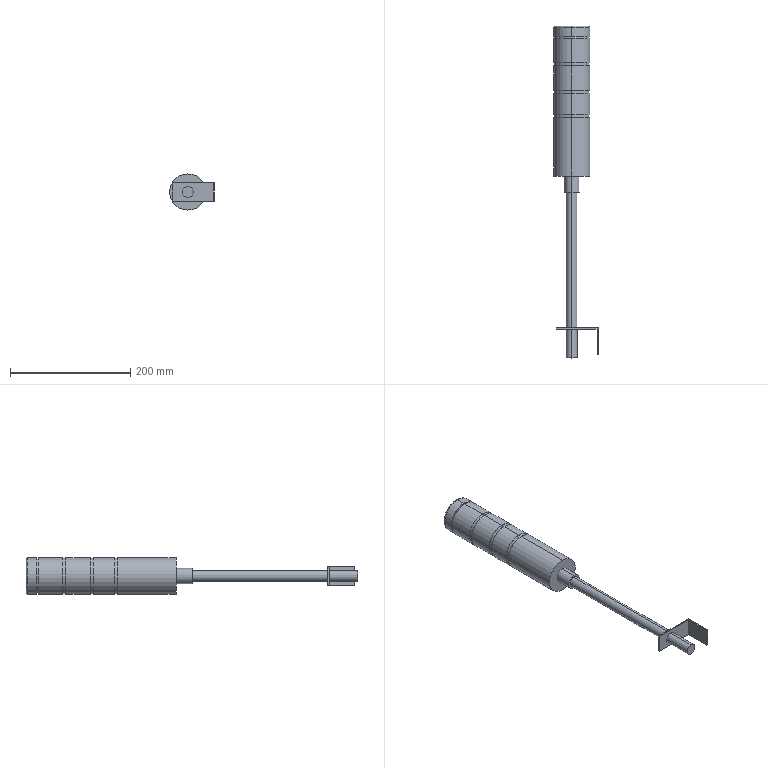Part | SolidWorks | features Boss 11, ICE 3, BossThin 1, Cut 1, Fillet 1, Shell 1, Sweep 1 | 1 solid | 46 faces | box 74 x 551.1 x 60 mm | volume 791689 mm3 | cylinder 24 | plane 20 | torus 2 | commonest cylinder face diameters 60 x10 59 x6 18 x4 25 x2 58 x2
STEP:
#1=CARTESIAN_POINT('',(212.5,682.5,-84.));
#2=VERTEX_POINT('',#1);
#3=CARTESIAN_POINT('',(212.5,682.5,-66.));
#4=VERTEX_POINT('',#3);
#5=CARTESIAN_POINT('',(212.5,682.5,-75.));
#6=DIRECTION('',(0.,-1.,0.));
#7=DIRECTION('',(0.,0.,-1.));
#8=AXIS2_PLACEMENT_3D('',#5,#6,#7);
#9=CIRCLE('',#8,9.);
#10=EDGE_CURVE('',#2,#4,#9,.T.);
#11=ORIENTED_EDGE('',*,*,#10,.F.);
#12=CARTESIAN_POINT('',(212.5,730.5,-84.));
#13=VERTEX_POINT('',#12);
#14=CARTESIAN_POINT('',(212.5,682.5,-84.));
#15=DIRECTION('',(0.,1.,0.));
#16=VECTOR('',#15,1000.);
#17=LINE('',#14,#16);
#18=EDGE_CURVE('',#2,#13,#17,.T.);
#19=ORIENTED_EDGE('',*,*,#18,.T.);
#20=CARTESIAN_POINT('',(212.5,730.5,-66.));
#21=VERTEX_POINT('',#20);
#22=CARTESIAN_POINT('',(212.5,730.5,-75.));
#23=DIRECTION('',(0.,1.,0.));
#24=DIRECTION('',(0.,0.,1.));
#25=AXIS2_PLACEMENT_3D('',#22,#23,#24);
#26=CIRCLE('',#25,9.);
#27=EDGE_CURVE('',#21,#13,#26,.T.);
#28=ORIENTED_EDGE('',*,*,#27,.F.);
#29=CARTESIAN_POINT('',(212.5,682.5,-66.));
#30=DIRECTION('',(0.,1.,0.));
#31=VECTOR('',#30,1000.);
#32=LINE('',#29,#31);
#33=EDGE_CURVE('',#4,#21,#32,.T.);
#34=ORIENTED_EDGE('',*,*,#33,.F.);
#35=EDGE_LOOP('',(#11,#19,#28,#34));
#36=FACE_OUTER_BOUND('',#35,.T.);
#37=CARTESIAN_POINT('',(212.5,682.5,-75.));
#38=DIRECTION('',(0.,1.,0.));
#39=DIRECTION('',(0.,0.,1.));
#40=AXIS2_PLACEMENT_3D('',#37,#38,#39);
#41=CYLINDRICAL_SURFACE('',#40,9.);
#42=ADVANCED_FACE('',(#36),#41,.T.);
#43=CARTESIAN_POINT('',(212.5,732.5,-66.));
#44=VERTEX_POINT('',#43);
#45=CARTESIAN_POINT('',(212.5,732.5,-84.));
#46=VERTEX_POINT('',#45);
#47=CARTESIAN_POINT('',(212.5,732.5,-75.));
#48=DIRECTION('',(0.,1.,0.));
#49=DIRECTION('',(0.,0.,1.));
#50=AXIS2_PLACEMENT_3D('',#47,#48,#49);
#51=CIRCLE('',#50,9.);
#52=EDGE_CURVE('',#44,#46,#51,.T.);
#53=ORIENTED_EDGE('',*,*,#52,.T.);
#54=CARTESIAN_POINT('',(212.5,957.5,-84.));
#55=VERTEX_POINT('',#54);
#56=CARTESIAN_POINT('',(212.5,682.5,-84.));
#57=DIRECTION('',(0.,1.,0.));
#58=VECTOR('',#57,1000.);
#59=LINE('',#56,#58);
#60=EDGE_CURVE('',#46,#55,#59,.T.);
#61=ORIENTED_EDGE('',*,*,#60,.T.);
#62=CARTESIAN_POINT('',(212.5,957.5,-66.));
#63=VERTEX_POINT('',#62);
#64=CARTESIAN_POINT('',(212.5,957.5,-75.));
#65=DIRECTION('',(0.,-1.,0.));
#66=DIRECTION('',(0.,0.,-1.));
#67=AXIS2_PLACEMENT_3D('',#64,#65,#66);
#68=CIRCLE('',#67,9.);
#69=EDGE_CURVE('',#55,#63,#68,.T.);
#70=ORIENTED_EDGE('',*,*,#69,.T.);
#71=CARTESIAN_POINT('',(212.5,682.5,-66.));
#72=DIRECTION('',(0.,1.,0.));
#73=VECTOR('',#72,1000.);
#74=LINE('',#71,#73);
#75=EDGE_CURVE('',#44,#63,#74,.T.);
#76=ORIENTED_EDGE('',*,*,#75,.F.);
#77=EDGE_LOOP('',(#53,#61,#70,#76));
#78=FACE_OUTER_BOUND('',#77,.T.);
#79=CARTESIAN_POINT('',(212.5,682.5,-75.));
#80=DIRECTION('',(0.,1.,0.));
#81=DIRECTION('',(0.,0.,1.));
#82=AXIS2_PLACEMENT_3D('',#79,#80,#81);
#83=CYLINDRICAL_SURFACE('',#82,9.);
#84=ADVANCED_FACE('',(#78),#83,.T.);
#85=CARTESIAN_POINT('',(212.5,957.5,-87.5));
#86=VERTEX_POINT('',#85);
#87=CARTESIAN_POINT('',(212.5,957.5,-62.5));
#88=VERTEX_POINT('',#87);
#89=CARTESIAN_POINT('',(212.5,957.5,-75.));
#90=DIRECTION('',(0.,-1.,0.));
#91=DIRECTION('',(0.,0.,-1.));
#92=AXIS2_PLACEMENT_3D('',#89,#90,#91);
#93=CIRCLE('',#92,12.5);
#94=EDGE_CURVE('',#86,#88,#93,.T.);
#95=ORIENTED_EDGE('',*,*,#94,.F.);
#96=CARTESIAN_POINT('',(212.5,984.5,-87.5));
#97=VERTEX_POINT('',#96);
#98=CARTESIAN_POINT('',(212.5,957.5,-87.5));
#99=DIRECTION('',(0.,1.,0.));
#100=VECTOR('',#99,1000.);
#101=LINE('',#98,#100);
#102=EDGE_CURVE('',#86,#97,#101,.T.);
#103=ORIENTED_EDGE('',*,*,#102,.T.);
#104=CARTESIAN_POINT('',(212.5,984.5,-62.5));
#105=VERTEX_POINT('',#104);
#106=CARTESIAN_POINT('',(212.5,984.5,-75.));
#107=DIRECTION('',(0.,-1.,0.));
#108=DIRECTION('',(0.,0.,1.));
#109=AXIS2_PLACEMENT_3D('',#106,#107,#108);
#110=CIRCLE('',#109,12.5);
#111=EDGE_CURVE('',#97,#105,#110,.T.);
#112=ORIENTED_EDGE('',*,*,#111,.T.);
#113=CARTESIAN_POINT('',(212.5,957.5,-62.5));
#114=DIRECTION('',(0.,1.,0.));
#115=VECTOR('',#114,1000.);
#116=LINE('',#113,#115);
#117=EDGE_CURVE('',#88,#105,#116,.T.);
#118=ORIENTED_EDGE('',*,*,#117,.F.);
#119=EDGE_LOOP('',(#95,#103,#112,#118));
#120=FACE_OUTER_BOUND('',#119,.T.);
#121=CARTESIAN_POINT('',(212.5,957.5,-75.));
#122=DIRECTION('',(0.,1.,0.));
#123=DIRECTION('',(0.,0.,1.));
#124=AXIS2_PLACEMENT_3D('',#121,#122,#123);
#125=CYLINDRICAL_SURFACE('',#124,12.5);
#126=ADVANCED_FACE('',(#120),#125,.T.);
#127=CARTESIAN_POINT('',(212.5,1230.6,-105.));
#128=VERTEX_POINT('',#127);
#129=CARTESIAN_POINT('',(212.5,1230.6,-45.));
#130=VERTEX_POINT('',#129);
#131=CARTESIAN_POINT('',(212.5,1230.6,-75.));
#132=DIRECTION('',(0.,-1.,0.));
#133=DIRECTION('',(0.,0.,1.));
#134=AXIS2_PLACEMENT_3D('',#131,#132,#133);
#135=CIRCLE('',#134,30.);
#136=EDGE_CURVE('',#128,#130,#135,.T.);
#137=ORIENTED_EDGE('',*,*,#136,.F.);
#138=CARTESIAN_POINT('',(212.5,1233.6,-102.));
#139=VERTEX_POINT('',#138);
#140=CARTESIAN_POINT('',(212.5,1230.6,-102.));
#141=DIRECTION('',(1.,0.,0.));
#142=DIRECTION('',(0.,0.,-1.));
#143=AXIS2_PLACEMENT_3D('',#140,#141,#142);
#144=CIRCLE('',#143,3.);
#145=EDGE_CURVE('',#128,#139,#144,.T.);
#146=ORIENTED_EDGE('',*,*,#145,.T.);
#147=CARTESIAN_POINT('',(212.5,1233.6,-48.));
#148=VERTEX_POINT('',#147);
#149=CARTESIAN_POINT('',(212.5,1233.6,-75.));
#150=DIRECTION('',(0.,1.,0.));
#151=DIRECTION('',(0.,0.,1.));
#152=AXIS2_PLACEMENT_3D('',#149,#150,#151);
#153=CIRCLE('',#152,27.);
#154=EDGE_CURVE('',#148,#139,#153,.T.);
#155=ORIENTED_EDGE('',*,*,#154,.F.);
#156=CARTESIAN_POINT('',(212.5,1230.6,-48.));
#157=DIRECTION('',(-1.,0.,0.));
#158=DIRECTION('',(0.,-1.,0.));
#159=AXIS2_PLACEMENT_3D('',#156,#157,#158);
#160=CIRCLE('',#159,3.);
#161=EDGE_CURVE('',#130,#148,#160,.T.);
#162=ORIENTED_EDGE('',*,*,#161,.F.);
#163=EDGE_LOOP('',(#137,#146,#155,#162));
#164=FACE_OUTER_BOUND('',#163,.T.);
#165=CARTESIAN_POINT('',(212.5,1230.6,-75.));
#166=DIRECTION('',(0.,1.,0.));
#167=DIRECTION('',(0.,0.,1.));
#168=AXIS2_PLACEMENT_3D('',#165,#166,#167);
#169=TOROIDAL_SURFACE('',#168,27.,3.);
#170=ADVANCED_FACE('',(#164),#169,.T.);
#171=ORIENTED_EDGE('',*,*,#136,.T.);
#172=CARTESIAN_POINT('',(212.5,1215.6,-45.));
#173=VERTEX_POINT('',#172);
#174=CARTESIAN_POINT('',(212.5,1233.6,-45.));
#175=DIRECTION('',(0.,-1.,0.));
#176=VECTOR('',#175,1000.);
#177=LINE('',#174,#176);
#178=EDGE_CURVE('',#130,#173,#177,.T.);
#179=ORIENTED_EDGE('',*,*,#178,.T.);
#180=CARTESIAN_POINT('',(212.5,1215.6,-105.));
#181=VERTEX_POINT('',#180);
#182=CARTESIAN_POINT('',(212.5,1215.6,-75.));
#183=DIRECTION('',(0.,1.,0.));
#184=DIRECTION('',(0.,0.,1.));
#185=AXIS2_PLACEMENT_3D('',#182,#183,#184);
#186=CIRCLE('',#185,30.);
#187=EDGE_CURVE('',#173,#181,#186,.T.);
#188=ORIENTED_EDGE('',*,*,#187,.T.);
#189=CARTESIAN_POINT('',(212.5,1233.6,-105.));
#190=DIRECTION('',(0.,-1.,0.));
#191=VECTOR('',#190,1000.);
#192=LINE('',#189,#191);
#193=EDGE_CURVE('',#128,#181,#192,.T.);
#194=ORIENTED_EDGE('',*,*,#193,.F.);
#195=EDGE_LOOP('',(#171,#179,#188,#194));
#196=FACE_OUTER_BOUND('',#195,.T.);
#197=CARTESIAN_POINT('',(212.5,1233.6,-75.));
#198=DIRECTION('',(0.,-1.,0.));
#199=DIRECTION('',(0.,0.,-1.));
#200=AXIS2_PLACEMENT_3D('',#197,#198,#199);
#201=CYLINDRICAL_SURFACE('',#200,30.);
#202=ADVANCED_FACE('',(#196),#201,.T.);
#203=CARTESIAN_POINT('',(212.5,1215.6,-46.));
#204=VERTEX_POINT('',#203);
#205=CARTESIAN_POINT('',(212.5,1215.6,-104.));
#206=VERTEX_POINT('',#205);
#207=CARTESIAN_POINT('',(212.5,1215.6,-75.));
#208=DIRECTION('',(0.,1.,0.));
#209=DIRECTION('',(0.,0.,1.));
#210=AXIS2_PLACEMENT_3D('',#207,#208,#209);
#211=CIRCLE('',#210,29.);
#212=EDGE_CURVE('',#204,#206,#211,.T.);
#213=ORIENTED_EDGE('',*,*,#212,.F.);
#214=CARTESIAN_POINT('',(212.5,1213.6,-46.));
#215=VERTEX_POINT('',#214);
#216=CARTESIAN_POINT('',(212.5,1215.6,-46.));
#217=DIRECTION('',(0.,-1.,0.));
#218=VECTOR('',#217,1000.);
#219=LINE('',#216,#218);
#220=EDGE_CURVE('',#204,#215,#219,.T.);
#221=ORIENTED_EDGE('',*,*,#220,.T.);
#222=CARTESIAN_POINT('',(212.5,1213.6,-104.));
#223=VERTEX_POINT('',#222);
#224=CARTESIAN_POINT('',(212.5,1213.6,-75.));
#225=DIRECTION('',(0.,1.,0.));
#226=DIRECTION('',(0.,0.,1.));
#227=AXIS2_PLACEMENT_3D('',#224,#225,#226);
#228=CIRCLE('',#227,29.);
#229=EDGE_CURVE('',#215,#223,#228,.T.);
#230=ORIENTED_EDGE('',*,*,#229,.T.);
#231=CARTESIAN_POINT('',(212.5,1215.6,-104.));
#232=DIRECTION('',(0.,-1.,0.));
#233=VECTOR('',#232,1000.);
#234=LINE('',#231,#233);
#235=EDGE_CURVE('',#206,#223,#234,.T.);
#236=ORIENTED_EDGE('',*,*,#235,.F.);
#237=EDGE_LOOP('',(#213,#221,#230,#236));
#238=FACE_OUTER_BOUND('',#237,.T.);
#239=CARTESIAN_POINT('',(212.5,1215.6,-75.));
#240=DIRECTION('',(0.,-1.,0.));
#241=DIRECTION('',(0.,0.,-1.));
#242=AXIS2_PLACEMENT_3D('',#239,#240,#241);
#243=CYLINDRICAL_SURFACE('',#242,29.);
#244=ADVANCED_FACE('',(#238),#243,.T.);
#245=CARTESIAN_POINT('',(212.5,1213.6,-45.));
#246=VERTEX_POINT('',#245);
#247=CARTESIAN_POINT('',(212.5,1213.6,-105.));
#248=VERTEX_POINT('',#247);
#249=CARTESIAN_POINT('',(212.5,1213.6,-75.));
#250=DIRECTION('',(0.,1.,0.));
#251=DIRECTION('',(0.,0.,1.));
#252=AXIS2_PLACEMENT_3D('',#249,#250,#251);
#253=CIRCLE('',#252,30.);
#254=EDGE_CURVE('',#246,#248,#253,.T.);
#255=ORIENTED_EDGE('',*,*,#254,.F.);
#256=CARTESIAN_POINT('',(212.5,1172.6,-45.));
#257=VERTEX_POINT('',#256);
#258=CARTESIAN_POINT('',(212.5,1213.6,-45.));
#259=DIRECTION('',(0.,-1.,0.));
#260=VECTOR('',#259,1000.);
#261=LINE('',#258,#260);
#262=EDGE_CURVE('',#246,#257,#261,.T.);
#263=ORIENTED_EDGE('',*,*,#262,.T.);
#264=CARTESIAN_POINT('',(212.5,1172.6,-105.));
#265=VERTEX_POINT('',#264);
#266=CARTESIAN_POINT('',(212.5,1172.6,-75.));
#267=DIRECTION('',(0.,1.,0.));
#268=DIRECTION('',(0.,0.,1.));
#269=AXIS2_PLACEMENT_3D('',#266,#267,#268);
#270=CIRCLE('',#269,30.);
#271=EDGE_CURVE('',#257,#265,#270,.T.);
#272=ORIENTED_EDGE('',*,*,#271,.T.);
#273=CARTESIAN_POINT('',(212.5,1213.6,-105.));
#274=DIRECTION('',(0.,-1.,0.));
#275=VECTOR('',#274,1000.);
#276=LINE('',#273,#275);
#277=EDGE_CURVE('',#248,#265,#276,.T.);
#278=ORIENTED_EDGE('',*,*,#277,.F.);
#279=EDGE_LOOP('',(#255,#263,#272,#278));
#280=FACE_OUTER_BOUND('',#279,.T.);
#281=CARTESIAN_POINT('',(212.5,1213.6,-75.));
#282=DIRECTION('',(0.,-1.,0.));
#283=DIRECTION('',(0.,0.,-1.));
#284=AXIS2_PLACEMENT_3D('',#281,#282,#283);
#285=CYLINDRICAL_SURFACE('',#284,30.);
#286=ADVANCED_FACE('',(#280),#285,.T.);
#287=CARTESIAN_POINT('',(212.5,1172.6,-45.5));
#288=VERTEX_POINT('',#287);
#289=CARTESIAN_POINT('',(212.5,1172.6,-104.5));
#290=VERTEX_POINT('',#289);
#291=CARTESIAN_POINT('',(212.5,1172.6,-75.));
#292=DIRECTION('',(0.,1.,0.));
#293=DIRECTION('',(0.,0.,1.));
#294=AXIS2_PLACEMENT_3D('',#291,#292,#293);
#295=CIRCLE('',#294,29.5);
#296=EDGE_CURVE('',#288,#290,#295,.T.);
#297=ORIENTED_EDGE('',*,*,#296,.F.);
#298=CARTESIAN_POINT('',(212.5,1167.6,-45.5));
#299=VERTEX_POINT('',#298);
#300=CARTESIAN_POINT('',(212.5,1172.6,-45.5));
#301=DIRECTION('',(0.,-1.,0.));
#302=VECTOR('',#301,1000.);
#303=LINE('',#300,#302);
#304=EDGE_CURVE('',#288,#299,#303,.T.);
#305=ORIENTED_EDGE('',*,*,#304,.T.);
#306=CARTESIAN_POINT('',(212.5,1167.6,-104.5));
#307=VERTEX_POINT('',#306);
#308=CARTESIAN_POINT('',(212.5,1167.6,-75.));
#309=DIRECTION('',(0.,1.,0.));
#310=DIRECTION('',(0.,0.,1.));
#311=AXIS2_PLACEMENT_3D('',#308,#309,#310);
#312=CIRCLE('',#311,29.5);
#313=EDGE_CURVE('',#299,#307,#312,.T.);
#314=ORIENTED_EDGE('',*,*,#313,.T.);
#315=CARTESIAN_POINT('',(212.5,1172.6,-104.5));
#316=DIRECTION('',(0.,-1.,0.));
#317=VECTOR('',#316,1000.);
#318=LINE('',#315,#317);
#319=EDGE_CURVE('',#290,#307,#318,.T.);
#320=ORIENTED_EDGE('',*,*,#319,.F.);
#321=EDGE_LOOP('',(#297,#305,#314,#320));
#322=FACE_OUTER_BOUND('',#321,.T.);
#323=CARTESIAN_POINT('',(212.5,1172.6,-75.));
#324=DIRECTION('',(0.,-1.,0.));
#325=DIRECTION('',(0.,0.,-1.));
#326=AXIS2_PLACEMENT_3D('',#323,#324,#325);
#327=CYLINDRICAL_SURFACE('',#326,29.5);
#328=ADVANCED_FACE('',(#322),#327,.T.);
#329=CARTESIAN_POINT('',(212.5,1167.6,-45.));
#330=VERTEX_POINT('',#329);
#331=CARTESIAN_POINT('',(212.5,1167.6,-105.));
#332=VERTEX_POINT('',#331);
#333=CARTESIAN_POINT('',(212.5,1167.6,-75.));
#334=DIRECTION('',(0.,1.,0.));
#335=DIRECTION('',(0.,0.,1.));
#336=AXIS2_PLACEMENT_3D('',#333,#334,#335);
#337=CIRCLE('',#336,30.);
#338=EDGE_CURVE('',#330,#332,#337,.T.);
#339=ORIENTED_EDGE('',*,*,#338,.F.);
#340=CARTESIAN_POINT('',(212.5,1126.6,-45.));
#341=VERTEX_POINT('',#340);
#342=CARTESIAN_POINT('',(212.5,1167.6,-45.));
#343=DIRECTION('',(0.,-1.,0.));
#344=VECTOR('',#343,1000.);
#345=LINE('',#342,#344);
#346=EDGE_CURVE('',#330,#341,#345,.T.);
#347=ORIENTED_EDGE('',*,*,#346,.T.);
#348=CARTESIAN_POINT('',(212.5,1126.6,-105.));
#349=VERTEX_POINT('',#348);
#350=CARTESIAN_POINT('',(212.5,1126.6,-75.));
#351=DIRECTION('',(0.,1.,0.));
#352=DIRECTION('',(0.,0.,1.));
#353=AXIS2_PLACEMENT_3D('',#350,#351,#352);
#354=CIRCLE('',#353,30.);
#355=EDGE_CURVE('',#341,#349,#354,.T.);
#356=ORIENTED_EDGE('',*,*,#355,.T.);
#357=CARTESIAN_POINT('',(212.5,1167.6,-105.));
#358=DIRECTION('',(0.,-1.,0.));
#359=VECTOR('',#358,1000.);
#360=LINE('',#357,#359);
#361=EDGE_CURVE('',#332,#349,#360,.T.);
#362=ORIENTED_EDGE('',*,*,#361,.F.);
#363=EDGE_LOOP('',(#339,#347,#356,#362));
#364=FACE_OUTER_BOUND('',#363,.T.);
#365=CARTESIAN_POINT('',(212.5,1167.6,-75.));
#366=DIRECTION('',(0.,-1.,0.));
#367=DIRECTION('',(0.,0.,-1.));
#368=AXIS2_PLACEMENT_3D('',#365,#366,#367);
#369=CYLINDRICAL_SURFACE('',#368,30.);
#370=ADVANCED_FACE('',(#364),#369,.T.);
#371=CARTESIAN_POINT('',(212.5,1126.6,-45.5));
#372=VERTEX_POINT('',#371);
#373=CARTESIAN_POINT('',(212.5,1126.6,-104.5));
#374=VERTEX_POINT('',#373);
#375=CARTESIAN_POINT('',(212.5,1126.6,-75.));
#376=DIRECTION('',(0.,1.,0.));
#377=DIRECTION('',(0.,0.,1.));
#378=AXIS2_PLACEMENT_3D('',#375,#376,#377);
#379=CIRCLE('',#378,29.5);
#380=EDGE_CURVE('',#372,#374,#379,.T.);
#381=ORIENTED_EDGE('',*,*,#380,.F.);
#382=CARTESIAN_POINT('',(212.5,1121.6,-45.5));
#383=VERTEX_POINT('',#382);
#384=CARTESIAN_POINT('',(212.5,1126.6,-45.5));
#385=DIRECTION('',(0.,-1.,0.));
#386=VECTOR('',#385,1000.);
#387=LINE('',#384,#386);
#388=EDGE_CURVE('',#372,#383,#387,.T.);
#389=ORIENTED_EDGE('',*,*,#388,.T.);
#390=CARTESIAN_POINT('',(212.5,1121.6,-104.5));
#391=VERTEX_POINT('',#390);
#392=CARTESIAN_POINT('',(212.5,1121.6,-75.));
#393=DIRECTION('',(0.,1.,0.));
#394=DIRECTION('',(0.,0.,1.));
#395=AXIS2_PLACEMENT_3D('',#392,#393,#394);
#396=CIRCLE('',#395,29.5);
#397=EDGE_CURVE('',#383,#391,#396,.T.);
#398=ORIENTED_EDGE('',*,*,#397,.T.);
#399=CARTESIAN_POINT('',(212.5,1126.6,-104.5));
#400=DIRECTION('',(0.,-1.,0.));
#401=VECTOR('',#400,1000.);
#402=LINE('',#399,#401);
#403=EDGE_CURVE('',#374,#391,#402,.T.);
#404=ORIENTED_EDGE('',*,*,#403,.F.);
#405=EDGE_LOOP('',(#381,#389,#398,#404));
#406=FACE_OUTER_BOUND('',#405,.T.);
#407=CARTESIAN_POINT('',(212.5,1126.6,-75.));
#408=DIRECTION('',(0.,-1.,0.));
#409=DIRECTION('',(0.,0.,-1.));
#410=AXIS2_PLACEMENT_3D('',#407,#408,#409);
#411=CYLINDRICAL_SURFACE('',#410,29.5);
#412=ADVANCED_FACE('',(#406),#411,.T.);
#413=CARTESIAN_POINT('',(212.5,1121.6,-45.));
#414=VERTEX_POINT('',#413);
#415=CARTESIAN_POINT('',(212.5,1121.6,-105.));
#416=VERTEX_POINT('',#415);
#417=CARTESIAN_POINT('',(212.5,1121.6,-75.));
#418=DIRECTION('',(0.,1.,0.));
#419=DIRECTION('',(0.,0.,1.));
#420=AXIS2_PLACEMENT_3D('',#417,#418,#419);
#421=CIRCLE('',#420,30.);
#422=EDGE_CURVE('',#414,#416,#421,.T.);
#423=ORIENTED_EDGE('',*,*,#422,.F.);
#424=CARTESIAN_POINT('',(212.5,1086.6,-45.));
#425=VERTEX_POINT('',#424);
#426=CARTESIAN_POINT('',(212.5,1121.6,-45.));
#427=DIRECTION('',(0.,-1.,0.));
#428=VECTOR('',#427,1000.);
#429=LINE('',#426,#428);
#430=EDGE_CURVE('',#414,#425,#429,.T.);
#431=ORIENTED_EDGE('',*,*,#430,.T.);
#432=CARTESIAN_POINT('',(212.5,1086.6,-105.));
#433=VERTEX_POINT('',#432);
#434=CARTESIAN_POINT('',(212.5,1086.6,-75.));
#435=DIRECTION('',(0.,1.,0.));
#436=DIRECTION('',(0.,0.,1.));
#437=AXIS2_PLACEMENT_3D('',#434,#435,#436);
#438=CIRCLE('',#437,30.);
#439=EDGE_CURVE('',#425,#433,#438,.T.);
#440=ORIENTED_EDGE('',*,*,#439,.T.);
#441=CARTESIAN_POINT('',(212.5,1121.6,-105.));
#442=DIRECTION('',(0.,-1.,0.));
#443=VECTOR('',#442,1000.);
#444=LINE('',#441,#443);
#445=EDGE_CURVE('',#416,#433,#444,.T.);
#446=ORIENTED_EDGE('',*,*,#445,.F.);
#447=EDGE_LOOP('',(#423,#431,#440,#446));
#448=FACE_OUTER_BOUND('',#447,.T.);
#449=CARTESIAN_POINT('',(212.5,1121.6,-75.));
#450=DIRECTION('',(0.,-1.,0.));
#451=DIRECTION('',(0.,0.,-1.));
#452=AXIS2_PLACEMENT_3D('',#449,#450,#451);
#453=CYLINDRICAL_SURFACE('',#452,30.);
#454=ADVANCED_FACE('',(#448),#453,.T.);
#455=CARTESIAN_POINT('',(212.5,1086.6,-45.5));
#456=VERTEX_POINT('',#455);
#457=CARTESIAN_POINT('',(212.5,1086.6,-104.5));
#458=VERTEX_POINT('',#457);
#459=CARTESIAN_POINT('',(212.5,1086.6,-75.));
#460=DIRECTION('',(0.,1.,0.));
#461=DIRECTION('',(0.,0.,1.));
#462=AXIS2_PLACEMENT_3D('',#459,#460,#461);
#463=CIRCLE('',#462,29.5);
#464=EDGE_CURVE('',#456,#458,#463,.T.);
#465=ORIENTED_EDGE('',*,*,#464,.F.);
#466=CARTESIAN_POINT('',(212.5,1081.6,-45.5));
#467=VERTEX_POINT('',#466);
#468=CARTESIAN_POINT('',(212.5,1086.6,-45.5));
#469=DIRECTION('',(0.,-1.,0.));
#470=VECTOR('',#469,1000.);
#471=LINE('',#468,#470);
#472=EDGE_CURVE('',#456,#467,#471,.T.);
#473=ORIENTED_EDGE('',*,*,#472,.T.);
#474=CARTESIAN_POINT('',(212.5,1081.6,-104.5));
#475=VERTEX_POINT('',#474);
#476=CARTESIAN_POINT('',(212.5,1081.6,-75.));
#477=DIRECTION('',(0.,1.,0.));
#478=DIRECTION('',(0.,0.,1.));
#479=AXIS2_PLACEMENT_3D('',#476,#477,#478);
#480=CIRCLE('',#479,29.5);
#481=EDGE_CURVE('',#467,#475,#480,.T.);
#482=ORIENTED_EDGE('',*,*,#481,.T.);
#483=CARTESIAN_POINT('',(212.5,1086.6,-104.5));
#484=DIRECTION('',(0.,-1.,0.));
#485=VECTOR('',#484,1000.);
#486=LINE('',#483,#485);
#487=EDGE_CURVE('',#458,#475,#486,.T.);
#488=ORIENTED_EDGE('',*,*,#487,.F.);
#489=EDGE_LOOP('',(#465,#473,#482,#488));
#490=FACE_OUTER_BOUND('',#489,.T.);
#491=CARTESIAN_POINT('',(212.5,1086.6,-75.));
#492=DIRECTION('',(0.,-1.,0.));
#493=DIRECTION('',(0.,0.,-1.));
#494=AXIS2_PLACEMENT_3D('',#491,#492,#493);
#495=CYLINDRICAL_SURFACE('',#494,29.5);
#496=ADVANCED_FACE('',(#490),#495,.T.);
#497=CARTESIAN_POINT('',(212.5,1081.6,-45.));
#498=VERTEX_POINT('',#497);
#499=CARTESIAN_POINT('',(212.5,1081.6,-105.));
#500=VERTEX_POINT('',#499);
#501=CARTESIAN_POINT('',(212.5,1081.6,-75.));
#502=DIRECTION('',(0.,1.,0.));
#503=DIRECTION('',(0.,0.,1.));
#504=AXIS2_PLACEMENT_3D('',#501,#502,#503);
#505=CIRCLE('',#504,30.);
#506=EDGE_CURVE('',#498,#500,#505,.T.);
#507=ORIENTED_EDGE('',*,*,#506,.F.);
#508=CARTESIAN_POINT('',(212.5,984.5,-45.));
#509=VERTEX_POINT('',#508);
#510=CARTESIAN_POINT('',(212.5,1081.6,-45.));
#511=DIRECTION('',(0.,-1.,0.));
#512=VECTOR('',#511,1000.);
#513=LINE('',#510,#512);
#514=EDGE_CURVE('',#498,#509,#513,.T.);
#515=ORIENTED_EDGE('',*,*,#514,.T.);
#516=CARTESIAN_POINT('',(212.5,984.5,-105.));
#517=VERTEX_POINT('',#516);
#518=CARTESIAN_POINT('',(212.5,984.5,-75.));
#519=DIRECTION('',(0.,1.,0.));
#520=DIRECTION('',(0.,0.,1.));
#521=AXIS2_PLACEMENT_3D('',#518,#519,#520);
#522=CIRCLE('',#521,30.);
#523=EDGE_CURVE('',#509,#517,#522,.T.);
#524=ORIENTED_EDGE('',*,*,#523,.T.);
#525=CARTESIAN_POINT('',(212.5,1081.6,-105.));
#526=DIRECTION('',(0.,-1.,0.));
#527=VECTOR('',#526,1000.);
#528=LINE('',#525,#527);
#529=EDGE_CURVE('',#500,#517,#528,.T.);
#530=ORIENTED_EDGE('',*,*,#529,.F.);
#531=EDGE_LOOP('',(#507,#515,#524,#530));
#532=FACE_OUTER_BOUND('',#531,.T.);
#533=CARTESIAN_POINT('',(212.5,1081.6,-75.));
#534=DIRECTION('',(0.,-1.,0.));
#535=DIRECTION('',(0.,0.,-1.));
#536=AXIS2_PLACEMENT_3D('',#533,#534,#535);
#537=CYLINDRICAL_SURFACE('',#536,30.);
#538=ADVANCED_FACE('',(#532),#537,.T.);
#539=CARTESIAN_POINT('',(212.5,957.5,-75.));
#540=DIRECTION('',(0.,-1.,0.));
#541=DIRECTION('',(0.,0.,-1.));
#542=AXIS2_PLACEMENT_3D('',#539,#540,#541);
#543=CIRCLE('',#542,12.5);
#544=EDGE_CURVE('',#88,#86,#543,.T.);
#545=ORIENTED_EDGE('',*,*,#544,.T.);
#546=ORIENTED_EDGE('',*,*,#94,.T.);
#547=EDGE_LOOP('',(#545,#546));
#548=FACE_OUTER_BOUND('',#547,.T.);
#549=CARTESIAN_POINT('',(212.5,957.5,-75.));
#550=DIRECTION('',(0.,-1.,0.));
#551=DIRECTION('',(0.,0.,-1.));
#552=AXIS2_PLACEMENT_3D('',#549,#550,#551);
#553=CIRCLE('',#552,9.);
#554=EDGE_CURVE('',#63,#55,#553,.T.);
#555=ORIENTED_EDGE('',*,*,#554,.F.);
#556=ORIENTED_EDGE('',*,*,#69,.F.);
#557=EDGE_LOOP('',(#555,#556));
#558=FACE_BOUND('',#557,.T.);
#559=CARTESIAN_POINT('',(212.5,957.5,-75.));
#560=DIRECTION('',(0.,-1.,0.));
#561=DIRECTION('',(0.,0.,-1.));
#562=AXIS2_PLACEMENT_3D('',#559,#560,#561);
#563=PLANE('',#562);
#564=ADVANCED_FACE('',(#548,#558),#563,.T.);
#565=CARTESIAN_POINT('',(212.5,984.5,-75.));
#566=DIRECTION('',(0.,1.,0.));
#567=DIRECTION('',(0.,0.,1.));
#568=AXIS2_PLACEMENT_3D('',#565,#566,#567);
#569=CIRCLE('',#568,30.);
#570=EDGE_CURVE('',#517,#509,#569,.T.);
#571=ORIENTED_EDGE('',*,*,#570,.F.);
#572=ORIENTED_EDGE('',*,*,#523,.F.);
#573=EDGE_LOOP('',(#571,#572));
#574=FACE_OUTER_BOUND('',#573,.T.);
#575=CARTESIAN_POINT('',(212.5,984.5,-75.));
#576=DIRECTION('',(0.,-1.,0.));
#577=DIRECTION('',(0.,0.,1.));
#578=AXIS2_PLACEMENT_3D('',#575,#576,#577);
#579=CIRCLE('',#578,12.5);
#580=EDGE_CURVE('',#105,#97,#579,.T.);
#581=ORIENTED_EDGE('',*,*,#580,.F.);
#582=ORIENTED_EDGE('',*,*,#111,.F.);
#583=EDGE_LOOP('',(#581,#582));
#584=FACE_BOUND('',#583,.T.);
#585=CARTESIAN_POINT('',(-24.,984.5,-125.));
#586=DIRECTION('',(0.,1.,0.));
#587=DIRECTION('',(0.,0.,1.));
#588=AXIS2_PLACEMENT_3D('',#585,#586,#587);
#589=PLANE('',#588);
#590=ADVANCED_FACE('',(#574,#584),#589,.F.);
#591=CARTESIAN_POINT('',(212.5,1213.6,-75.));
#592=DIRECTION('',(0.,1.,0.));
#593=DIRECTION('',(0.,0.,1.));
#594=AXIS2_PLACEMENT_3D('',#591,#592,#593);
#595=CIRCLE('',#594,30.);
#596=EDGE_CURVE('',#248,#246,#595,.T.);
#597=ORIENTED_EDGE('',*,*,#596,.T.);
#598=ORIENTED_EDGE('',*,*,#254,.T.);
#599=EDGE_LOOP('',(#597,#598));
#600=FACE_OUTER_BOUND('',#599,.T.);
#601=CARTESIAN_POINT('',(212.5,1213.6,-75.));
#602=DIRECTION('',(0.,1.,0.));
#603=DIRECTION('',(0.,0.,1.));
#604=AXIS2_PLACEMENT_3D('',#601,#602,#603);
#605=CIRCLE('',#604,29.);
#606=EDGE_CURVE('',#223,#215,#605,.T.);
#607=ORIENTED_EDGE('',*,*,#606,.F.);
#608=ORIENTED_EDGE('',*,*,#229,.F.);
#609=EDGE_LOOP('',(#607,#608));
#610=FACE_BOUND('',#609,.T.);
#611=CARTESIAN_POINT('',(212.5,1213.6,-75.));
#612=DIRECTION('',(0.,1.,0.));
#613=DIRECTION('',(0.,0.,1.));
#614=AXIS2_PLACEMENT_3D('',#611,#612,#613);
#615=PLANE('',#614);
#616=ADVANCED_FACE('',(#600,#610),#615,.T.);
#617=CARTESIAN_POINT('',(212.5,1167.6,-75.));
#618=DIRECTION('',(0.,1.,0.));
#619=DIRECTION('',(0.,0.,1.));
#620=AXIS2_PLACEMENT_3D('',#617,#618,#619);
#621=CIRCLE('',#620,30.);
#622=EDGE_CURVE('',#332,#330,#621,.T.);
#623=ORIENTED_EDGE('',*,*,#622,.T.);
#624=ORIENTED_EDGE('',*,*,#338,.T.);
#625=EDGE_LOOP('',(#623,#624));
#626=FACE_OUTER_BOUND('',#625,.T.);
#627=CARTESIAN_POINT('',(212.5,1167.6,-75.));
#628=DIRECTION('',(0.,1.,0.));
#629=DIRECTION('',(0.,0.,1.));
#630=AXIS2_PLACEMENT_3D('',#627,#628,#629);
#631=CIRCLE('',#630,29.5);
#632=EDGE_CURVE('',#307,#299,#631,.T.);
#633=ORIENTED_EDGE('',*,*,#632,.F.);
#634=ORIENTED_EDGE('',*,*,#313,.F.);
#635=EDGE_LOOP('',(#633,#634));
#636=FACE_BOUND('',#635,.T.);
#637=CARTESIAN_POINT('',(212.5,1167.6,-75.));
#638=DIRECTION('',(0.,1.,0.));
#639=DIRECTION('',(0.,0.,1.));
#640=AXIS2_PLACEMENT_3D('',#637,#638,#639);
#641=PLANE('',#640);
#642=ADVANCED_FACE('',(#626,#636),#641,.T.);
#643=CARTESIAN_POINT('',(212.5,1121.6,-75.));
#644=DIRECTION('',(0.,1.,0.));
#645=DIRECTION('',(0.,0.,1.));
#646=AXIS2_PLACEMENT_3D('',#643,#644,#645);
#647=CIRCLE('',#646,30.);
#648=EDGE_CURVE('',#416,#414,#647,.T.);
#649=ORIENTED_EDGE('',*,*,#648,.T.);
#650=ORIENTED_EDGE('',*,*,#422,.T.);
#651=EDGE_LOOP('',(#649,#650));
#652=FACE_OUTER_BOUND('',#651,.T.);
#653=CARTESIAN_POINT('',(212.5,1121.6,-75.));
#654=DIRECTION('',(0.,1.,0.));
#655=DIRECTION('',(0.,0.,1.));
#656=AXIS2_PLACEMENT_3D('',#653,#654,#655);
#657=CIRCLE('',#656,29.5);
#658=EDGE_CURVE('',#391,#383,#657,.T.);
#659=ORIENTED_EDGE('',*,*,#658,.F.);
#660=ORIENTED_EDGE('',*,*,#397,.F.);
#661=EDGE_LOOP('',(#659,#660));
#662=FACE_BOUND('',#661,.T.);
#663=CARTESIAN_POINT('',(212.5,1121.6,-75.));
#664=DIRECTION('',(0.,1.,0.));
#665=DIRECTION('',(0.,0.,1.));
#666=AXIS2_PLACEMENT_3D('',#663,#664,#665);
#667=PLANE('',#666);
#668=ADVANCED_FACE('',(#652,#662),#667,.T.);
#669=CARTESIAN_POINT('',(212.5,1081.6,-75.));
#670=DIRECTION('',(0.,1.,0.));
#671=DIRECTION('',(0.,0.,1.));
#672=AXIS2_PLACEMENT_3D('',#669,#670,#671);
#673=CIRCLE('',#672,30.);
#674=EDGE_CURVE('',#500,#498,#673,.T.);
#675=ORIENTED_EDGE('',*,*,#674,.T.);
#676=ORIENTED_EDGE('',*,*,#506,.T.);
#677=EDGE_LOOP('',(#675,#676));
#678=FACE_OUTER_BOUND('',#677,.T.);
#679=CARTESIAN_POINT('',(212.5,1081.6,-75.));
#680=DIRECTION('',(0.,1.,0.));
#681=DIRECTION('',(0.,0.,1.));
#682=AXIS2_PLACEMENT_3D('',#679,#680,#681);
#683=CIRCLE('',#682,29.5);
#684=EDGE_CURVE('',#475,#467,#683,.T.);
#685=ORIENTED_EDGE('',*,*,#684,.F.);
#686=ORIENTED_EDGE('',*,*,#481,.F.);
#687=EDGE_LOOP('',(#685,#686));
#688=FACE_BOUND('',#687,.T.);
#689=CARTESIAN_POINT('',(212.5,1081.6,-75.));
#690=DIRECTION('',(0.,1.,0.));
#691=DIRECTION('',(0.,0.,1.));
#692=AXIS2_PLACEMENT_3D('',#689,#690,#691);
#693=PLANE('',#692);
#694=ADVANCED_FACE('',(#678,#688),#693,.T.);
#695=ORIENTED_EDGE('',*,*,#514,.F.);
#696=ORIENTED_EDGE('',*,*,#674,.F.);
#697=ORIENTED_EDGE('',*,*,#529,.T.);
#698=ORIENTED_EDGE('',*,*,#570,.T.);
#699=EDGE_LOOP('',(#695,#696,#697,#698));
#700=FACE_OUTER_BOUND('',#699,.T.);
#701=CARTESIAN_POINT('',(212.5,1081.6,-75.));
#702=DIRECTION('',(0.,-1.,0.));
#703=DIRECTION('',(0.,0.,-1.));
#704=AXIS2_PLACEMENT_3D('',#701,#702,#703);
#705=CYLINDRICAL_SURFACE('',#704,30.);
#706=ADVANCED_FACE('',(#700),#705,.T.);
#707=ORIENTED_EDGE('',*,*,#472,.F.);
#708=CARTESIAN_POINT('',(212.5,1086.6,-75.));
#709=DIRECTION('',(0.,1.,0.));
#710=DIRECTION('',(0.,0.,1.));
#711=AXIS2_PLACEMENT_3D('',#708,#709,#710);
#712=CIRCLE('',#711,29.5);
#713=EDGE_CURVE('',#458,#456,#712,.T.);
#714=ORIENTED_EDGE('',*,*,#713,.F.);
#715=ORIENTED_EDGE('',*,*,#487,.T.);
#716=ORIENTED_EDGE('',*,*,#684,.T.);
#717=EDGE_LOOP('',(#707,#714,#715,#716));
#718=FACE_OUTER_BOUND('',#717,.T.);
#719=CARTESIAN_POINT('',(212.5,1086.6,-75.));
#720=DIRECTION('',(0.,-1.,0.));
#721=DIRECTION('',(0.,0.,-1.));
#722=AXIS2_PLACEMENT_3D('',#719,#720,#721);
#723=CYLINDRICAL_SURFACE('',#722,29.5);
#724=ADVANCED_FACE('',(#718),#723,.T.);
#725=CARTESIAN_POINT('',(212.5,1086.6,-75.));
#726=DIRECTION('',(0.,1.,0.));
#727=DIRECTION('',(0.,0.,1.));
#728=AXIS2_PLACEMENT_3D('',#725,#726,#727);
#729=CIRCLE('',#728,30.);
#730=EDGE_CURVE('',#433,#425,#729,.T.);
#731=ORIENTED_EDGE('',*,*,#730,.F.);
#732=ORIENTED_EDGE('',*,*,#439,.F.);
#733=EDGE_LOOP('',(#731,#732));
#734=FACE_OUTER_BOUND('',#733,.T.);
#735=ORIENTED_EDGE('',*,*,#713,.T.);
#736=ORIENTED_EDGE('',*,*,#464,.T.);
#737=EDGE_LOOP('',(#735,#736));
#738=FACE_BOUND('',#737,.T.);
#739=CARTESIAN_POINT('',(212.5,1086.6,-75.));
#740=DIRECTION('',(0.,1.,0.));
#741=DIRECTION('',(0.,0.,1.));
#742=AXIS2_PLACEMENT_3D('',#739,#740,#741);
#743=PLANE('',#742);
#744=ADVANCED_FACE('',(#734,#738),#743,.F.);
#745=ORIENTED_EDGE('',*,*,#430,.F.);
#746=ORIENTED_EDGE('',*,*,#648,.F.);
#747=ORIENTED_EDGE('',*,*,#445,.T.);
#748=ORIENTED_EDGE('',*,*,#730,.T.);
#749=EDGE_LOOP('',(#745,#746,#747,#748));
#750=FACE_OUTER_BOUND('',#749,.T.);
#751=CARTESIAN_POINT('',(212.5,1121.6,-75.));
#752=DIRECTION('',(0.,-1.,0.));
#753=DIRECTION('',(0.,0.,-1.));
#754=AXIS2_PLACEMENT_3D('',#751,#752,#753);
#755=CYLINDRICAL_SURFACE('',#754,30.);
#756=ADVANCED_FACE('',(#750),#755,.T.);
#757=ORIENTED_EDGE('',*,*,#388,.F.);
#758=CARTESIAN_POINT('',(212.5,1126.6,-75.));
#759=DIRECTION('',(0.,1.,0.));
#760=DIRECTION('',(0.,0.,1.));
#761=AXIS2_PLACEMENT_3D('',#758,#759,#760);
#762=CIRCLE('',#761,29.5);
#763=EDGE_CURVE('',#374,#372,#762,.T.);
#764=ORIENTED_EDGE('',*,*,#763,.F.);
#765=ORIENTED_EDGE('',*,*,#403,.T.);
#766=ORIENTED_EDGE('',*,*,#658,.T.);
#767=EDGE_LOOP('',(#757,#764,#765,#766));
#768=FACE_OUTER_BOUND('',#767,.T.);
#769=CARTESIAN_POINT('',(212.5,1126.6,-75.));
#770=DIRECTION('',(0.,-1.,0.));
#771=DIRECTION('',(0.,0.,-1.));
#772=AXIS2_PLACEMENT_3D('',#769,#770,#771);
#773=CYLINDRICAL_SURFACE('',#772,29.5);
#774=ADVANCED_FACE('',(#768),#773,.T.);
#775=CARTESIAN_POINT('',(212.5,1126.6,-75.));
#776=DIRECTION('',(0.,1.,0.));
#777=DIRECTION('',(0.,0.,1.));
#778=AXIS2_PLACEMENT_3D('',#775,#776,#777);
#779=CIRCLE('',#778,30.);
#780=EDGE_CURVE('',#349,#341,#779,.T.);
#781=ORIENTED_EDGE('',*,*,#780,.F.);
#782=ORIENTED_EDGE('',*,*,#355,.F.);
#783=EDGE_LOOP('',(#781,#782));
#784=FACE_OUTER_BOUND('',#783,.T.);
#785=ORIENTED_EDGE('',*,*,#763,.T.);
#786=ORIENTED_EDGE('',*,*,#380,.T.);
#787=EDGE_LOOP('',(#785,#786));
#788=FACE_BOUND('',#787,.T.);
#789=CARTESIAN_POINT('',(212.5,1126.6,-75.));
#790=DIRECTION('',(0.,1.,0.));
#791=DIRECTION('',(0.,0.,1.));
#792=AXIS2_PLACEMENT_3D('',#789,#790,#791);
#793=PLANE('',#792);
#794=ADVANCED_FACE('',(#784,#788),#793,.F.);
#795=ORIENTED_EDGE('',*,*,#346,.F.);
#796=ORIENTED_EDGE('',*,*,#622,.F.);
#797=ORIENTED_EDGE('',*,*,#361,.T.);
#798=ORIENTED_EDGE('',*,*,#780,.T.);
#799=EDGE_LOOP('',(#795,#796,#797,#798));
#800=FACE_OUTER_BOUND('',#799,.T.);
#801=CARTESIAN_POINT('',(212.5,1167.6,-75.));
#802=DIRECTION('',(0.,-1.,0.));
#803=DIRECTION('',(0.,0.,-1.));
#804=AXIS2_PLACEMENT_3D('',#801,#802,#803);
#805=CYLINDRICAL_SURFACE('',#804,30.);
#806=ADVANCED_FACE('',(#800),#805,.T.);
#807=ORIENTED_EDGE('',*,*,#304,.F.);
#808=CARTESIAN_POINT('',(212.5,1172.6,-75.));
#809=DIRECTION('',(0.,1.,0.));
#810=DIRECTION('',(0.,0.,1.));
#811=AXIS2_PLACEMENT_3D('',#808,#809,#810);
#812=CIRCLE('',#811,29.5);
#813=EDGE_CURVE('',#290,#288,#812,.T.);
#814=ORIENTED_EDGE('',*,*,#813,.F.);
#815=ORIENTED_EDGE('',*,*,#319,.T.);
#816=ORIENTED_EDGE('',*,*,#632,.T.);
#817=EDGE_LOOP('',(#807,#814,#815,#816));
#818=FACE_OUTER_BOUND('',#817,.T.);
#819=CARTESIAN_POINT('',(212.5,1172.6,-75.));
#820=DIRECTION('',(0.,-1.,0.));
#821=DIRECTION('',(0.,0.,-1.));
#822=AXIS2_PLACEMENT_3D('',#819,#820,#821);
#823=CYLINDRICAL_SURFACE('',#822,29.5);
#824=ADVANCED_FACE('',(#818),#823,.T.);
#825=CARTESIAN_POINT('',(212.5,1172.6,-75.));
#826=DIRECTION('',(0.,1.,0.));
#827=DIRECTION('',(0.,0.,1.));
#828=AXIS2_PLACEMENT_3D('',#825,#826,#827);
#829=CIRCLE('',#828,30.);
#830=EDGE_CURVE('',#265,#257,#829,.T.);
#831=ORIENTED_EDGE('',*,*,#830,.F.);
#832=ORIENTED_EDGE('',*,*,#271,.F.);
#833=EDGE_LOOP('',(#831,#832));
#834=FACE_OUTER_BOUND('',#833,.T.);
#835=ORIENTED_EDGE('',*,*,#813,.T.);
#836=ORIENTED_EDGE('',*,*,#296,.T.);
#837=EDGE_LOOP('',(#835,#836));
#838=FACE_BOUND('',#837,.T.);
#839=CARTESIAN_POINT('',(212.5,1172.6,-75.));
#840=DIRECTION('',(0.,1.,0.));
#841=DIRECTION('',(0.,0.,1.));
#842=AXIS2_PLACEMENT_3D('',#839,#840,#841);
#843=PLANE('',#842);
#844=ADVANCED_FACE('',(#834,#838),#843,.F.);
#845=ORIENTED_EDGE('',*,*,#262,.F.);
#846=ORIENTED_EDGE('',*,*,#596,.F.);
#847=ORIENTED_EDGE('',*,*,#277,.T.);
#848=ORIENTED_EDGE('',*,*,#830,.T.);
#849=EDGE_LOOP('',(#845,#846,#847,#848));
#850=FACE_OUTER_BOUND('',#849,.T.);
#851=CARTESIAN_POINT('',(212.5,1213.6,-75.));
#852=DIRECTION('',(0.,-1.,0.));
#853=DIRECTION('',(0.,0.,-1.));
#854=AXIS2_PLACEMENT_3D('',#851,#852,#853);
#855=CYLINDRICAL_SURFACE('',#854,30.);
#856=ADVANCED_FACE('',(#850),#855,.T.);
#857=ORIENTED_EDGE('',*,*,#220,.F.);
#858=CARTESIAN_POINT('',(212.5,1215.6,-75.));
#859=DIRECTION('',(0.,1.,0.));
#860=DIRECTION('',(0.,0.,1.));
#861=AXIS2_PLACEMENT_3D('',#858,#859,#860);
#862=CIRCLE('',#861,29.);
#863=EDGE_CURVE('',#206,#204,#862,.T.);
#864=ORIENTED_EDGE('',*,*,#863,.F.);
#865=ORIENTED_EDGE('',*,*,#235,.T.);
#866=ORIENTED_EDGE('',*,*,#606,.T.);
#867=EDGE_LOOP('',(#857,#864,#865,#866));
#868=FACE_OUTER_BOUND('',#867,.T.);
#869=CARTESIAN_POINT('',(212.5,1215.6,-75.));
#870=DIRECTION('',(0.,-1.,0.));
#871=DIRECTION('',(0.,0.,-1.));
#872=AXIS2_PLACEMENT_3D('',#869,#870,#871);
#873=CYLINDRICAL_SURFACE('',#872,29.);
#874=ADVANCED_FACE('',(#868),#873,.T.);
#875=CARTESIAN_POINT('',(212.5,1215.6,-75.));
#876=DIRECTION('',(0.,1.,0.));
#877=DIRECTION('',(0.,0.,1.));
#878=AXIS2_PLACEMENT_3D('',#875,#876,#877);
#879=CIRCLE('',#878,30.);
#880=EDGE_CURVE('',#181,#173,#879,.T.);
#881=ORIENTED_EDGE('',*,*,#880,.F.);
#882=ORIENTED_EDGE('',*,*,#187,.F.);
#883=EDGE_LOOP('',(#881,#882));
#884=FACE_OUTER_BOUND('',#883,.T.);
#885=ORIENTED_EDGE('',*,*,#863,.T.);
#886=ORIENTED_EDGE('',*,*,#212,.T.);
#887=EDGE_LOOP('',(#885,#886));
#888=FACE_BOUND('',#887,.T.);
#889=CARTESIAN_POINT('',(212.5,1215.6,-75.));
#890=DIRECTION('',(0.,1.,0.));
#891=DIRECTION('',(0.,0.,1.));
#892=AXIS2_PLACEMENT_3D('',#889,#890,#891);
#893=PLANE('',#892);
#894=ADVANCED_FACE('',(#884,#888),#893,.F.);
#895=ORIENTED_EDGE('',*,*,#178,.F.);
#896=CARTESIAN_POINT('',(212.5,1230.6,-75.));
#897=DIRECTION('',(0.,-1.,0.));
#898=DIRECTION('',(0.,0.,1.));
#899=AXIS2_PLACEMENT_3D('',#896,#897,#898);
#900=CIRCLE('',#899,30.);
#901=EDGE_CURVE('',#130,#128,#900,.T.);
#902=ORIENTED_EDGE('',*,*,#901,.T.);
#903=ORIENTED_EDGE('',*,*,#193,.T.);
#904=ORIENTED_EDGE('',*,*,#880,.T.);
#905=EDGE_LOOP('',(#895,#902,#903,#904));
#906=FACE_OUTER_BOUND('',#905,.T.);
#907=CARTESIAN_POINT('',(212.5,1233.6,-75.));
#908=DIRECTION('',(0.,-1.,0.));
#909=DIRECTION('',(0.,0.,-1.));
#910=AXIS2_PLACEMENT_3D('',#907,#908,#909);
#911=CYLINDRICAL_SURFACE('',#910,30.);
#912=ADVANCED_FACE('',(#906),#911,.T.);
#913=ORIENTED_EDGE('',*,*,#154,.T.);
#914=CARTESIAN_POINT('',(212.5,1233.6,-75.));
#915=DIRECTION('',(0.,1.,0.));
#916=DIRECTION('',(0.,0.,1.));
#917=AXIS2_PLACEMENT_3D('',#914,#915,#916);
#918=CIRCLE('',#917,27.);
#919=EDGE_CURVE('',#139,#148,#918,.T.);
#920=ORIENTED_EDGE('',*,*,#919,.T.);
#921=EDGE_LOOP('',(#913,#920));
#922=FACE_OUTER_BOUND('',#921,.T.);
#923=CARTESIAN_POINT('',(212.5,1233.6,-75.));
#924=DIRECTION('',(0.,1.,0.));
#925=DIRECTION('',(0.,0.,1.));
#926=AXIS2_PLACEMENT_3D('',#923,#924,#925);
#927=PLANE('',#926);
#928=ADVANCED_FACE('',(#922),#927,.T.);
#929=ORIENTED_EDGE('',*,*,#145,.F.);
#930=ORIENTED_EDGE('',*,*,#901,.F.);
#931=ORIENTED_EDGE('',*,*,#161,.T.);
#932=ORIENTED_EDGE('',*,*,#919,.F.);
#933=EDGE_LOOP('',(#929,#930,#931,#932));
#934=FACE_OUTER_BOUND('',#933,.T.);
#935=CARTESIAN_POINT('',(212.5,1230.6,-75.));
#936=DIRECTION('',(0.,1.,0.));
#937=DIRECTION('',(0.,0.,1.));
#938=AXIS2_PLACEMENT_3D('',#935,#936,#937);
#939=TOROIDAL_SURFACE('',#938,27.,3.);
#940=ADVANCED_FACE('',(#934),#939,.T.);
#941=ORIENTED_EDGE('',*,*,#102,.F.);
#942=ORIENTED_EDGE('',*,*,#544,.F.);
#943=ORIENTED_EDGE('',*,*,#117,.T.);
#944=ORIENTED_EDGE('',*,*,#580,.T.);
#945=EDGE_LOOP('',(#941,#942,#943,#944));
#946=FACE_OUTER_BOUND('',#945,.T.);
#947=CARTESIAN_POINT('',(212.5,957.5,-75.));
#948=DIRECTION('',(0.,1.,0.));
#949=DIRECTION('',(0.,0.,1.));
#950=AXIS2_PLACEMENT_3D('',#947,#948,#949);
#951=CYLINDRICAL_SURFACE('',#950,12.5);
#952=ADVANCED_FACE('',(#946),#951,.T.);
#953=ORIENTED_EDGE('',*,*,#60,.F.);
#954=CARTESIAN_POINT('',(212.5,732.5,-75.));
#955=DIRECTION('',(0.,1.,0.));
#956=DIRECTION('',(0.,0.,1.));
#957=AXIS2_PLACEMENT_3D('',#954,#955,#956);
#958=CIRCLE('',#957,9.);
#959=EDGE_CURVE('',#46,#44,#958,.T.);
#960=ORIENTED_EDGE('',*,*,#959,.T.);
#961=ORIENTED_EDGE('',*,*,#75,.T.);
#962=ORIENTED_EDGE('',*,*,#554,.T.);
#963=EDGE_LOOP('',(#953,#960,#961,#962));
#964=FACE_OUTER_BOUND('',#963,.T.);
#965=CARTESIAN_POINT('',(212.5,682.5,-75.));
#966=DIRECTION('',(0.,1.,0.));
#967=DIRECTION('',(0.,0.,1.));
#968=AXIS2_PLACEMENT_3D('',#965,#966,#967);
#969=CYLINDRICAL_SURFACE('',#968,9.);
#970=ADVANCED_FACE('',(#964),#969,.T.);
#971=CARTESIAN_POINT('',(186.5,732.5,-90.));
#972=VERTEX_POINT('',#971);
#973=CARTESIAN_POINT('',(256.5,732.5,-90.));
#974=VERTEX_POINT('',#973);
#975=CARTESIAN_POINT('',(186.5,732.5,-90.));
#976=DIRECTION('',(1.,0.,0.));
#977=VECTOR('',#976,1000.);
#978=LINE('',#975,#977);
#979=EDGE_CURVE('',#972,#974,#978,.T.);
#980=ORIENTED_EDGE('',*,*,#979,.F.);
#981=CARTESIAN_POINT('',(186.5,732.5,-60.));
#982=VERTEX_POINT('',#981);
#983=CARTESIAN_POINT('',(186.5,732.5,-60.));
#984=DIRECTION('',(0.,0.,-1.));
#985=VECTOR('',#984,1000.);
#986=LINE('',#983,#985);
#987=EDGE_CURVE('',#982,#972,#986,.T.);
#988=ORIENTED_EDGE('',*,*,#987,.F.);
#989=CARTESIAN_POINT('',(256.5,732.5,-60.));
#990=VERTEX_POINT('',#989);
#991=CARTESIAN_POINT('',(186.5,732.5,-60.));
#992=DIRECTION('',(1.,0.,0.));
#993=VECTOR('',#992,1000.);
#994=LINE('',#991,#993);
#995=EDGE_CURVE('',#982,#990,#994,.T.);
#996=ORIENTED_EDGE('',*,*,#995,.T.);
#997=CARTESIAN_POINT('',(256.5,732.5,-60.));
#998=DIRECTION('',(0.,0.,-1.));
#999=VECTOR('',#998,1000.);
#1000=LINE('',#997,#999);
#1001=EDGE_CURVE('',#990,#974,#1000,.T.);
#1002=ORIENTED_EDGE('',*,*,#1001,.T.);
#1003=EDGE_LOOP('',(#980,#988,#996,#1002));
#1004=FACE_OUTER_BOUND('',#1003,.T.);
#1005=ORIENTED_EDGE('',*,*,#52,.F.);
#1006=ORIENTED_EDGE('',*,*,#959,.F.);
#1007=EDGE_LOOP('',(#1005,#1006));
#1008=FACE_BOUND('',#1007,.T.);
#1009=CARTESIAN_POINT('',(186.5,732.5,-60.));
#1010=DIRECTION('',(0.,1.,0.));
#1011=DIRECTION('',(0.,0.,1.));
#1012=AXIS2_PLACEMENT_3D('',#1009,#1010,#1011);
#1013=PLANE('',#1012);
#1014=ADVANCED_FACE('',(#1004,#1008),#1013,.T.);
#1015=CARTESIAN_POINT('',(186.5,730.5,-90.));
#1016=VERTEX_POINT('',#1015);
#1017=CARTESIAN_POINT('',(254.5,730.5,-90.));
#1018=VERTEX_POINT('',#1017);
#1019=CARTESIAN_POINT('',(186.5,730.5,-90.));
#1020=DIRECTION('',(1.,0.,0.));
#1021=VECTOR('',#1020,1000.);
#1022=LINE('',#1019,#1021);
#1023=EDGE_CURVE('',#1016,#1018,#1022,.T.);
#1024=ORIENTED_EDGE('',*,*,#1023,.T.);
#1025=CARTESIAN_POINT('',(254.5,730.5,-60.));
#1026=VERTEX_POINT('',#1025);
#1027=CARTESIAN_POINT('',(254.5,730.5,-60.));
#1028=DIRECTION('',(0.,0.,-1.));
#1029=VECTOR('',#1028,1000.);
#1030=LINE('',#1027,#1029);
#1031=EDGE_CURVE('',#1026,#1018,#1030,.T.);
#1032=ORIENTED_EDGE('',*,*,#1031,.F.);
#1033=CARTESIAN_POINT('',(186.5,730.5,-60.));
#1034=VERTEX_POINT('',#1033);
#1035=CARTESIAN_POINT('',(186.5,730.5,-60.));
#1036=DIRECTION('',(1.,0.,0.));
#1037=VECTOR('',#1036,1000.);
#1038=LINE('',#1035,#1037);
#1039=EDGE_CURVE('',#1034,#1026,#1038,.T.);
#1040=ORIENTED_EDGE('',*,*,#1039,.F.);
#1041=CARTESIAN_POINT('',(186.5,730.5,-60.));
#1042=DIRECTION('',(0.,0.,-1.));
#1043=VECTOR('',#1042,1000.);
#1044=LINE('',#1041,#1043);
#1045=EDGE_CURVE('',#1034,#1016,#1044,.T.);
#1046=ORIENTED_EDGE('',*,*,#1045,.T.);
#1047=EDGE_LOOP('',(#1024,#1032,#1040,#1046));
#1048=FACE_OUTER_BOUND('',#1047,.T.);
#1049=ORIENTED_EDGE('',*,*,#27,.T.);
#1050=CARTESIAN_POINT('',(212.5,730.5,-75.));
#1051=DIRECTION('',(0.,1.,0.));
#1052=DIRECTION('',(0.,0.,1.));
#1053=AXIS2_PLACEMENT_3D('',#1050,#1051,#1052);
#1054=CIRCLE('',#1053,9.);
#1055=EDGE_CURVE('',#13,#21,#1054,.T.);
#1056=ORIENTED_EDGE('',*,*,#1055,.T.);
#1057=EDGE_LOOP('',(#1049,#1056));
#1058=FACE_BOUND('',#1057,.T.);
#1059=CARTESIAN_POINT('',(186.5,730.5,-60.));
#1060=DIRECTION('',(0.,1.,0.));
#1061=DIRECTION('',(0.,0.,1.));
#1062=AXIS2_PLACEMENT_3D('',#1059,#1060,#1061);
#1063=PLANE('',#1062);
#1064=ADVANCED_FACE('',(#1048,#1058),#1063,.F.);
#1065=CARTESIAN_POINT('',(254.5,687.5,-90.));
#1066=VERTEX_POINT('',#1065);
#1067=CARTESIAN_POINT('',(254.5,732.5,-90.));
#1068=DIRECTION('',(0.,-1.,0.));
#1069=VECTOR('',#1068,1000.);
#1070=LINE('',#1067,#1069);
#1071=EDGE_CURVE('',#1018,#1066,#1070,.T.);
#1072=ORIENTED_EDGE('',*,*,#1071,.T.);
#1073=CARTESIAN_POINT('',(254.5,687.5,-60.));
#1074=VERTEX_POINT('',#1073);
#1075=CARTESIAN_POINT('',(254.5,687.5,-60.));
#1076=DIRECTION('',(0.,0.,-1.));
#1077=VECTOR('',#1076,1000.);
#1078=LINE('',#1075,#1077);
#1079=EDGE_CURVE('',#1074,#1066,#1078,.T.);
#1080=ORIENTED_EDGE('',*,*,#1079,.F.);
#1081=CARTESIAN_POINT('',(254.5,732.5,-60.));
#1082=DIRECTION('',(0.,-1.,0.));
#1083=VECTOR('',#1082,1000.);
#1084=LINE('',#1081,#1083);
#1085=EDGE_CURVE('',#1026,#1074,#1084,.T.);
#1086=ORIENTED_EDGE('',*,*,#1085,.F.);
#1087=ORIENTED_EDGE('',*,*,#1031,.T.);
#1088=EDGE_LOOP('',(#1072,#1080,#1086,#1087));
#1089=FACE_OUTER_BOUND('',#1088,.T.);
#1090=CARTESIAN_POINT('',(254.5,732.5,-60.));
#1091=DIRECTION('',(1.,0.,0.));
#1092=DIRECTION('',(0.,0.,-1.));
#1093=AXIS2_PLACEMENT_3D('',#1090,#1091,#1092);
#1094=PLANE('',#1093);
#1095=ADVANCED_FACE('',(#1089),#1094,.F.);
#1096=CARTESIAN_POINT('',(256.5,687.5,-90.));
#1097=VERTEX_POINT('',#1096);
#1098=CARTESIAN_POINT('',(256.5,687.5,-90.));
#1099=DIRECTION('',(-1.,0.,0.));
#1100=VECTOR('',#1099,1000.);
#1101=LINE('',#1098,#1100);
#1102=EDGE_CURVE('',#1097,#1066,#1101,.T.);
#1103=ORIENTED_EDGE('',*,*,#1102,.F.);
#1104=CARTESIAN_POINT('',(256.5,687.5,-60.));
#1105=VERTEX_POINT('',#1104);
#1106=CARTESIAN_POINT('',(256.5,687.5,-60.));
#1107=DIRECTION('',(0.,0.,-1.));
#1108=VECTOR('',#1107,1000.);
#1109=LINE('',#1106,#1108);
#1110=EDGE_CURVE('',#1105,#1097,#1109,.T.);
#1111=ORIENTED_EDGE('',*,*,#1110,.F.);
#1112=CARTESIAN_POINT('',(256.5,687.5,-60.));
#1113=DIRECTION('',(-1.,0.,0.));
#1114=VECTOR('',#1113,1000.);
#1115=LINE('',#1112,#1114);
#1116=EDGE_CURVE('',#1105,#1074,#1115,.T.);
#1117=ORIENTED_EDGE('',*,*,#1116,.T.);
#1118=ORIENTED_EDGE('',*,*,#1079,.T.);
#1119=EDGE_LOOP('',(#1103,#1111,#1117,#1118));
#1120=FACE_OUTER_BOUND('',#1119,.T.);
#1121=CARTESIAN_POINT('',(256.5,687.5,-60.));
#1122=DIRECTION('',(0.,-1.,0.));
#1123=DIRECTION('',(0.,0.,-1.));
#1124=AXIS2_PLACEMENT_3D('',#1121,#1122,#1123);
#1125=PLANE('',#1124);
#1126=ADVANCED_FACE('',(#1120),#1125,.T.);
#1127=CARTESIAN_POINT('',(256.5,732.5,-90.));
#1128=DIRECTION('',(0.,-1.,0.));
#1129=VECTOR('',#1128,1000.);
#1130=LINE('',#1127,#1129);
#1131=EDGE_CURVE('',#974,#1097,#1130,.T.);
#1132=ORIENTED_EDGE('',*,*,#1131,.F.);
#1133=ORIENTED_EDGE('',*,*,#1001,.F.);
#1134=CARTESIAN_POINT('',(256.5,732.5,-60.));
#1135=DIRECTION('',(0.,-1.,0.));
#1136=VECTOR('',#1135,1000.);
#1137=LINE('',#1134,#1136);
#1138=EDGE_CURVE('',#990,#1105,#1137,.T.);
#1139=ORIENTED_EDGE('',*,*,#1138,.T.);
#1140=ORIENTED_EDGE('',*,*,#1110,.T.);
#1141=EDGE_LOOP('',(#1132,#1133,#1139,#1140));
#1142=FACE_OUTER_BOUND('',#1141,.T.);
#1143=CARTESIAN_POINT('',(256.5,732.5,-60.));
#1144=DIRECTION('',(1.,0.,0.));
#1145=DIRECTION('',(0.,0.,-1.));
#1146=AXIS2_PLACEMENT_3D('',#1143,#1144,#1145);
#1147=PLANE('',#1146);
#1148=ADVANCED_FACE('',(#1142),#1147,.T.);
#1149=CARTESIAN_POINT('',(186.5,730.5,-90.));
#1150=DIRECTION('',(0.,1.,0.));
#1151=VECTOR('',#1150,1000.);
#1152=LINE('',#1149,#1151);
#1153=EDGE_CURVE('',#1016,#972,#1152,.T.);
#1154=ORIENTED_EDGE('',*,*,#1153,.F.);
#1155=ORIENTED_EDGE('',*,*,#1045,.F.);
#1156=CARTESIAN_POINT('',(186.5,730.5,-60.));
#1157=DIRECTION('',(0.,1.,0.));
#1158=VECTOR('',#1157,1000.);
#1159=LINE('',#1156,#1158);
#1160=EDGE_CURVE('',#1034,#982,#1159,.T.);
#1161=ORIENTED_EDGE('',*,*,#1160,.T.);
#1162=ORIENTED_EDGE('',*,*,#987,.T.);
#1163=EDGE_LOOP('',(#1154,#1155,#1161,#1162));
#1164=FACE_OUTER_BOUND('',#1163,.T.);
#1165=CARTESIAN_POINT('',(186.5,730.5,-60.));
#1166=DIRECTION('',(-1.,0.,0.));
#1167=DIRECTION('',(0.,0.,1.));
#1168=AXIS2_PLACEMENT_3D('',#1165,#1166,#1167);
#1169=PLANE('',#1168);
#1170=ADVANCED_FACE('',(#1164),#1169,.T.);
#1171=ORIENTED_EDGE('',*,*,#1085,.T.);
#1172=ORIENTED_EDGE('',*,*,#1116,.F.);
#1173=ORIENTED_EDGE('',*,*,#1138,.F.);
#1174=ORIENTED_EDGE('',*,*,#995,.F.);
#1175=ORIENTED_EDGE('',*,*,#1160,.F.);
#1176=ORIENTED_EDGE('',*,*,#1039,.T.);
#1177=EDGE_LOOP('',(#1171,#1172,#1173,#1174,#1175,#1176));
#1178=FACE_OUTER_BOUND('',#1177,.T.);
#1179=CARTESIAN_POINT('',(254.5,687.5,-60.));
#1180=DIRECTION('',(0.,0.,1.));
#1181=DIRECTION('',(1.,0.,0.));
#1182=AXIS2_PLACEMENT_3D('',#1179,#1180,#1181);
#1183=PLANE('',#1182);
#1184=ADVANCED_FACE('',(#1178),#1183,.T.);
#1185=ORIENTED_EDGE('',*,*,#1071,.F.);
#1186=ORIENTED_EDGE('',*,*,#1023,.F.);
#1187=ORIENTED_EDGE('',*,*,#1153,.T.);
#1188=ORIENTED_EDGE('',*,*,#979,.T.);
#1189=ORIENTED_EDGE('',*,*,#1131,.T.);
#1190=ORIENTED_EDGE('',*,*,#1102,.T.);
#1191=EDGE_LOOP('',(#1185,#1186,#1187,#1188,#1189,#1190));
#1192=FACE_OUTER_BOUND('',#1191,.T.);
#1193=CARTESIAN_POINT('',(254.5,687.5,-90.));
#1194=DIRECTION('',(0.,0.,1.));
#1195=DIRECTION('',(1.,0.,0.));
#1196=AXIS2_PLACEMENT_3D('',#1193,#1194,#1195);
#1197=PLANE('',#1196);
#1198=ADVANCED_FACE('',(#1192),#1197,.F.);
#1199=CARTESIAN_POINT('',(212.5,682.5,-75.));
#1200=DIRECTION('',(0.,-1.,0.));
#1201=DIRECTION('',(0.,0.,-1.));
#1202=AXIS2_PLACEMENT_3D('',#1199,#1200,#1201);
#1203=CIRCLE('',#1202,9.);
#1204=EDGE_CURVE('',#4,#2,#1203,.T.);
#1205=ORIENTED_EDGE('',*,*,#1204,.T.);
#1206=ORIENTED_EDGE('',*,*,#10,.T.);
#1207=EDGE_LOOP('',(#1205,#1206));
#1208=FACE_OUTER_BOUND('',#1207,.T.);
#1209=CARTESIAN_POINT('',(212.5,682.5,-75.));
#1210=DIRECTION('',(0.,-1.,0.));
#1211=DIRECTION('',(0.,0.,-1.));
#1212=AXIS2_PLACEMENT_3D('',#1209,#1210,#1211);
#1213=PLANE('',#1212);
#1214=ADVANCED_FACE('',(#1208),#1213,.T.);
#1215=ORIENTED_EDGE('',*,*,#18,.F.);
#1216=ORIENTED_EDGE('',*,*,#1204,.F.);
#1217=ORIENTED_EDGE('',*,*,#33,.T.);
#1218=ORIENTED_EDGE('',*,*,#1055,.F.);
#1219=EDGE_LOOP('',(#1215,#1216,#1217,#1218));
#1220=FACE_OUTER_BOUND('',#1219,.T.);
#1221=CARTESIAN_POINT('',(212.5,682.5,-75.));
#1222=DIRECTION('',(0.,1.,0.));
#1223=DIRECTION('',(0.,0.,1.));
#1224=AXIS2_PLACEMENT_3D('',#1221,#1222,#1223);
#1225=CYLINDRICAL_SURFACE('',#1224,9.);
#1226=ADVANCED_FACE('',(#1220),#1225,.T.);
#1227=CLOSED_SHELL('',(#42,#84,#126,#170,#202,#244,#286,#328,#370,#412,#454,#496,#538,#564,#590,#616,#642,#668,#694,#706,#724,#744,#756,#774,#794,#806,#824,#844,#856,#874,#894,#912,#928,#940,#952,#970,#1014,#1064,#1095,#1126,#1148,#1170,#1184,#1198,#1214,#1226));
#1228=MANIFOLD_SOLID_BREP('',#1227);
#1229=CARTESIAN_POINT('',(0.,0.,0.));
#1230=DIRECTION('',(0.,0.,1.));
#1231=DIRECTION('',(1.,0.,0.));
#1232=AXIS2_PLACEMENT_3D('',#1229,#1230,#1231);
#1233=(LENGTH_UNIT()NAMED_UNIT(*)SI_UNIT(.MILLI.,.METRE.));
#1234=UNCERTAINTY_MEASURE_WITH_UNIT(LENGTH_MEASURE(0.00001),#1233,'','');
#1235=(NAMED_UNIT(*)PLANE_ANGLE_UNIT()SI_UNIT($,.RADIAN.));
#1236=(NAMED_UNIT(*)SI_UNIT($,.STERADIAN.)SOLID_ANGLE_UNIT());
#1237=(GEOMETRIC_REPRESENTATION_CONTEXT(3)GLOBAL_UNCERTAINTY_ASSIGNED_CONTEXT((#1234))GLOBAL_UNIT_ASSIGNED_CONTEXT((#1233,#1235,#1236))REPRESENTATION_CONTEXT('',''));
#1238=ADVANCED_BREP_SHAPE_REPRESENTATION('',(#1228,#1232),#1237);